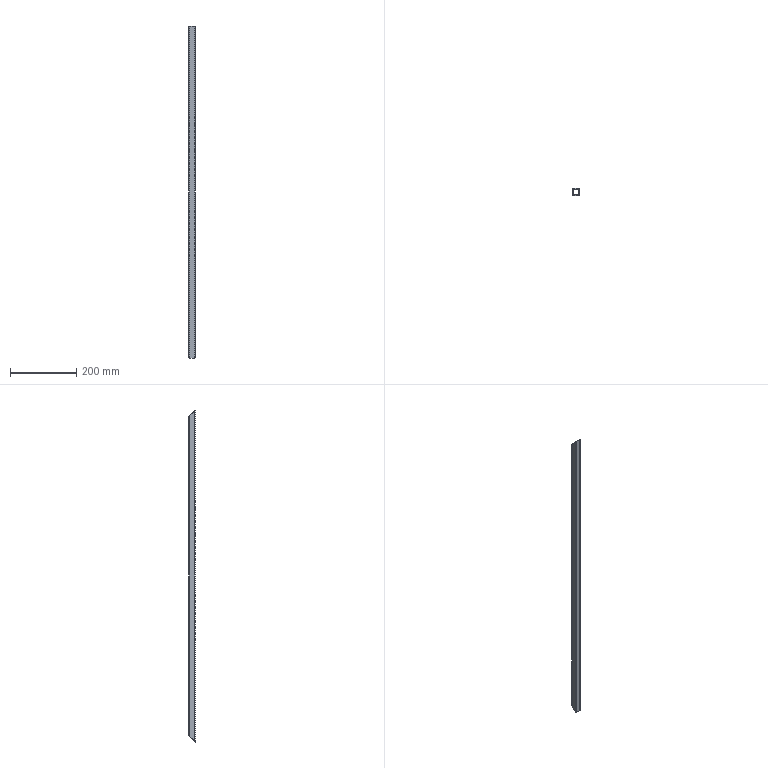Part | STEP file | 1 | 1 solid | 18 faces | box 20 x 20 x 1000 mm | volume 136914 mm3 | plane 10 | cylinder 8 | commonest cylinder face diameters 4 x4 6 x4